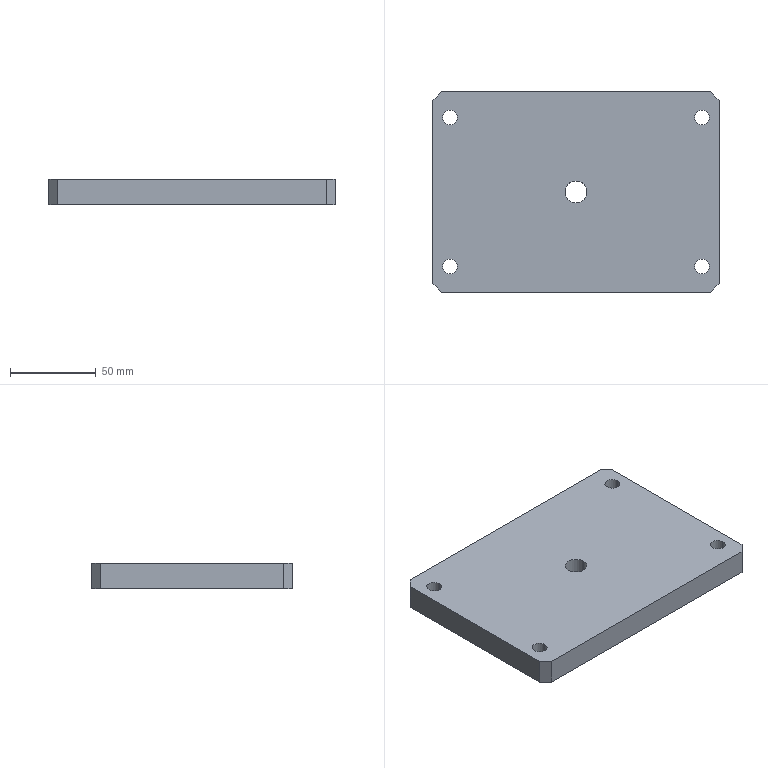Part | STEP file | Cylinder pad plate | 1 solid | 20 faces | box 167 x 117 x 14.75 mm | volume 282156 mm3 | cylinder 10 | plane 10 | commonest cylinder face diameters 8.6 x8 12.738 x2